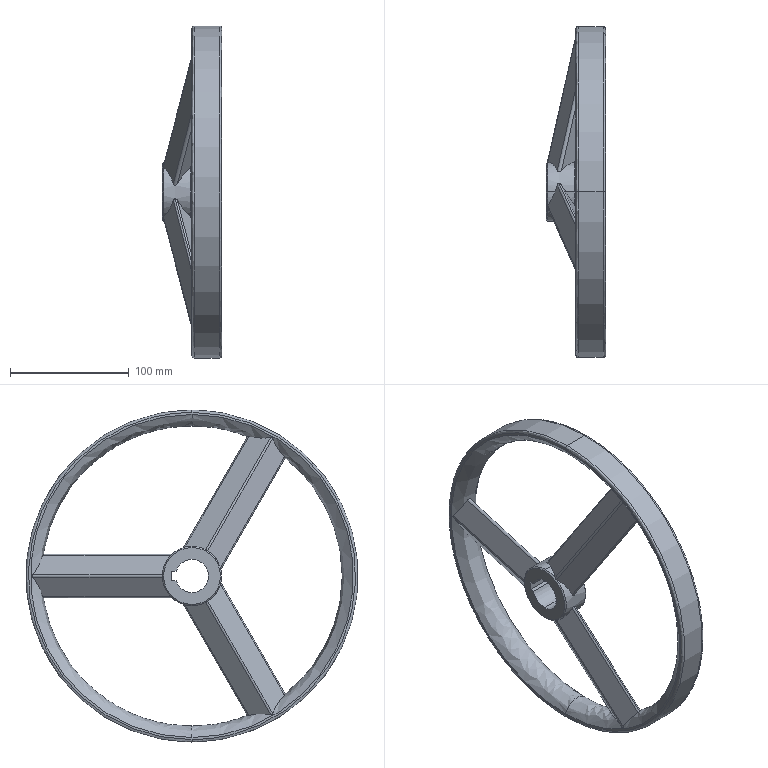Part | SolidWorks | features BaseBody 2 | 2 solids | 57 faces | box 50 x 280 x 280 mm | volume 423489 mm3 | cylinder 25 | plane 19 | spline 9 | cone 4 | commonest cylinder face diameters 4 x15 50 x5 28 x3 280 x2